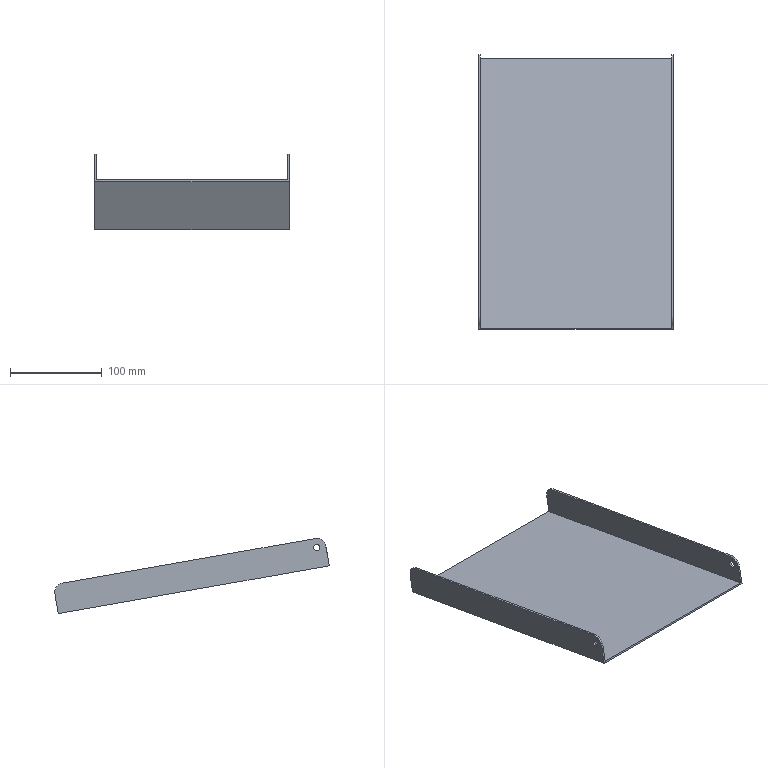Part | NX | features HB 2 | 1 solid | 16 faces | box 213 x 300.028 x 82.132 mm | volume 163815 mm3 | plane 10 | cylinder 6 | commonest cylinder face diameters 20 x4 7 x2
STEP:
#1=CARTESIAN_POINT('',(3721.,686.06,-368.904));
#2=VERTEX_POINT('',#1);
#3=CARTESIAN_POINT('',(3721.,686.966,-372.285));
#4=DIRECTION('',(1.,0.,0.));
#5=DIRECTION('',(0.,-0.2588,0.9659));
#6=AXIS2_PLACEMENT_3D('',#3,#4,#5);
#7=CIRCLE('',#6,3.5);
#8=EDGE_CURVE('',#2,#2,#7,.T.);
#9=ORIENTED_EDGE('',*,*,#8,.T.);
#10=EDGE_LOOP('',(#9));
#11=FACE_BOUND('',#10,.T.);
#12=CARTESIAN_POINT('',(3719.,686.06,-368.904));
#13=VERTEX_POINT('',#12);
#14=CARTESIAN_POINT('',(3719.,686.966,-372.285));
#15=DIRECTION('',(-1.,0.,0.));
#16=DIRECTION('',(0.,-0.2588,0.9659));
#17=AXIS2_PLACEMENT_3D('',#14,#15,#16);
#18=CIRCLE('',#17,3.5);
#19=EDGE_CURVE('',#13,#13,#18,.T.);
#20=ORIENTED_EDGE('',*,*,#19,.T.);
#21=EDGE_LOOP('',(#20));
#22=FACE_BOUND('',#21,.T.);
#23=CARTESIAN_POINT('',(2999.,686.966,-372.285));
#24=DIRECTION('',(1.,0.,0.));
#25=DIRECTION('',(0.,0.2588,-0.9659));
#26=AXIS2_PLACEMENT_3D('',#23,#24,#25);
#27=CYLINDRICAL_SURFACE('',#26,3.5);
#28=ADVANCED_FACE('',(#11,#22),#27,.F.);
#29=CARTESIAN_POINT('',(3721.,965.062,-411.167));
#30=VERTEX_POINT('',#29);
#31=CARTESIAN_POINT('',(3721.,688.702,-362.437));
#32=VERTEX_POINT('',#31);
#33=CARTESIAN_POINT('',(3721.,564.245,-340.492));
#34=DIRECTION('',(0.,-0.9848,0.1736));
#35=VECTOR('',#34,1000.);
#36=LINE('',#33,#35);
#37=EDGE_CURVE('',#30,#32,#36,.T.);
#38=ORIENTED_EDGE('',*,*,#37,.F.);
#39=CARTESIAN_POINT('',(3719.,965.062,-411.167));
#40=VERTEX_POINT('',#39);
#41=CARTESIAN_POINT('',(3605.,965.062,-411.167));
#42=DIRECTION('',(1.,0.,0.));
#43=VECTOR('',#42,1000.);
#44=LINE('',#41,#43);
#45=EDGE_CURVE('',#40,#30,#44,.T.);
#46=ORIENTED_EDGE('',*,*,#45,.F.);
#47=CARTESIAN_POINT('',(3719.,688.702,-362.437));
#48=VERTEX_POINT('',#47);
#49=CARTESIAN_POINT('',(3719.,564.245,-340.492));
#50=DIRECTION('',(0.,-0.9848,0.1736));
#51=VECTOR('',#50,1000.);
#52=LINE('',#49,#51);
#53=EDGE_CURVE('',#40,#48,#52,.T.);
#54=ORIENTED_EDGE('',*,*,#53,.T.);
#55=CARTESIAN_POINT('',(3605.,688.702,-362.437));
#56=DIRECTION('',(1.,0.,0.));
#57=VECTOR('',#56,1000.);
#58=LINE('',#55,#57);
#59=EDGE_CURVE('',#48,#32,#58,.T.);
#60=ORIENTED_EDGE('',*,*,#59,.T.);
#61=EDGE_LOOP('',(#38,#46,#54,#60));
#62=FACE_BOUND('',#61,.T.);
#63=CARTESIAN_POINT('',(3605.,564.245,-340.492));
#64=DIRECTION('',(0.,-0.1736,-0.9848));
#65=DIRECTION('',(0.,0.9848,-0.1736));
#66=AXIS2_PLACEMENT_3D('',#63,#64,#65);
#67=PLANE('',#66);
#68=ADVANCED_FACE('',(#62),#67,.F.);
#69=CARTESIAN_POINT('',(3721.,973.174,-422.751));
#70=VERTEX_POINT('',#69);
#71=CARTESIAN_POINT('',(3721.,963.326,-421.015));
#72=DIRECTION('',(-1.,0.,0.));
#73=DIRECTION('',(0.,-0.2588,0.9659));
#74=AXIS2_PLACEMENT_3D('',#71,#72,#73);
#75=CIRCLE('',#74,10.);
#76=EDGE_CURVE('',#30,#70,#75,.T.);
#77=ORIENTED_EDGE('',*,*,#76,.T.);
#78=CARTESIAN_POINT('',(3719.,973.174,-422.751));
#79=VERTEX_POINT('',#78);
#80=CARTESIAN_POINT('',(3605.,973.174,-422.751));
#81=DIRECTION('',(-1.,0.,0.));
#82=VECTOR('',#81,1000.);
#83=LINE('',#80,#82);
#84=EDGE_CURVE('',#70,#79,#83,.T.);
#85=ORIENTED_EDGE('',*,*,#84,.T.);
#86=CARTESIAN_POINT('',(3719.,963.326,-421.015));
#87=DIRECTION('',(1.,0.,0.));
#88=DIRECTION('',(0.,-0.2588,0.9659));
#89=AXIS2_PLACEMENT_3D('',#86,#87,#88);
#90=CIRCLE('',#89,10.);
#91=EDGE_CURVE('',#79,#40,#90,.T.);
#92=ORIENTED_EDGE('',*,*,#91,.T.);
#93=ORIENTED_EDGE('',*,*,#45,.T.);
#94=EDGE_LOOP('',(#77,#85,#92,#93));
#95=FACE_BOUND('',#94,.T.);
#96=CARTESIAN_POINT('',(3605.,963.326,-421.015));
#97=DIRECTION('',(-1.,0.,0.));
#98=DIRECTION('',(0.,-0.2588,0.9659));
#99=AXIS2_PLACEMENT_3D('',#96,#97,#98);
#100=CYLINDRICAL_SURFACE('',#99,10.);
#101=ADVANCED_FACE('',(#95),#100,.T.);
#102=ORIENTED_EDGE('',*,*,#53,.F.);
#103=ORIENTED_EDGE('',*,*,#91,.F.);
#104=CARTESIAN_POINT('',(3719.,969.354,-444.417));
#105=VERTEX_POINT('',#104);
#106=CARTESIAN_POINT('',(3719.,969.701,-442.448));
#107=DIRECTION('',(0.,0.1736,0.9848));
#108=VECTOR('',#107,1000.);
#109=LINE('',#106,#108);
#110=EDGE_CURVE('',#105,#79,#109,.T.);
#111=ORIENTED_EDGE('',*,*,#110,.F.);
#112=CARTESIAN_POINT('',(3719.,673.298,-392.215));
#113=VERTEX_POINT('',#112);
#114=CARTESIAN_POINT('',(3719.,558.689,-372.006));
#115=DIRECTION('',(0.,0.9848,-0.1736));
#116=VECTOR('',#115,1000.);
#117=LINE('',#114,#116);
#118=EDGE_CURVE('',#113,#105,#117,.T.);
#119=ORIENTED_EDGE('',*,*,#118,.F.);
#120=CARTESIAN_POINT('',(3719.,677.118,-370.549));
#121=VERTEX_POINT('',#120);
#122=CARTESIAN_POINT('',(3719.,673.645,-390.245));
#123=DIRECTION('',(0.,0.1736,0.9848));
#124=VECTOR('',#123,1000.);
#125=LINE('',#122,#124);
#126=EDGE_CURVE('',#113,#121,#125,.T.);
#127=ORIENTED_EDGE('',*,*,#126,.T.);
#128=CARTESIAN_POINT('',(3719.,686.966,-372.285));
#129=DIRECTION('',(-1.,0.,0.));
#130=DIRECTION('',(0.,0.5736,0.8192));
#131=AXIS2_PLACEMENT_3D('',#128,#129,#130);
#132=CIRCLE('',#131,10.);
#133=EDGE_CURVE('',#121,#48,#132,.T.);
#134=ORIENTED_EDGE('',*,*,#133,.T.);
#135=EDGE_LOOP('',(#102,#103,#111,#119,#127,#134));
#136=FACE_BOUND('',#135,.T.);
#137=ORIENTED_EDGE('',*,*,#19,.F.);
#138=EDGE_LOOP('',(#137));
#139=FACE_BOUND('',#138,.T.);
#140=CARTESIAN_POINT('',(3719.,559.036,-370.036));
#141=DIRECTION('',(1.,0.,0.));
#142=DIRECTION('',(0.,0.2588,-0.9659));
#143=AXIS2_PLACEMENT_3D('',#140,#141,#142);
#144=PLANE('',#143);
#145=ADVANCED_FACE('',(#136,#139),#144,.F.);
#146=CARTESIAN_POINT('',(3721.,677.118,-370.549));
#147=VERTEX_POINT('',#146);
#148=CARTESIAN_POINT('',(3721.,686.966,-372.285));
#149=DIRECTION('',(1.,0.,0.));
#150=DIRECTION('',(0.,0.5736,0.8192));
#151=AXIS2_PLACEMENT_3D('',#148,#149,#150);
#152=CIRCLE('',#151,10.);
#153=EDGE_CURVE('',#32,#147,#152,.T.);
#154=ORIENTED_EDGE('',*,*,#153,.F.);
#155=ORIENTED_EDGE('',*,*,#59,.F.);
#156=ORIENTED_EDGE('',*,*,#133,.F.);
#157=CARTESIAN_POINT('',(3700.,677.118,-370.549));
#158=DIRECTION('',(-1.,0.,0.));
#159=VECTOR('',#158,1000.);
#160=LINE('',#157,#159);
#161=EDGE_CURVE('',#147,#121,#160,.T.);
#162=ORIENTED_EDGE('',*,*,#161,.F.);
#163=EDGE_LOOP('',(#154,#155,#156,#162));
#164=FACE_BOUND('',#163,.T.);
#165=CARTESIAN_POINT('',(3605.,686.966,-372.285));
#166=DIRECTION('',(-1.,0.,0.));
#167=DIRECTION('',(0.,0.5736,0.8192));
#168=AXIS2_PLACEMENT_3D('',#165,#166,#167);
#169=CYLINDRICAL_SURFACE('',#168,10.);
#170=ADVANCED_FACE('',(#164),#169,.T.);
#171=ORIENTED_EDGE('',*,*,#76,.F.);
#172=ORIENTED_EDGE('',*,*,#37,.T.);
#173=ORIENTED_EDGE('',*,*,#153,.T.);
#174=CARTESIAN_POINT('',(3721.,673.645,-390.245));
#175=VERTEX_POINT('',#174);
#176=CARTESIAN_POINT('',(3721.,673.645,-390.245));
#177=DIRECTION('',(0.,0.1736,0.9848));
#178=VECTOR('',#177,1000.);
#179=LINE('',#176,#178);
#180=EDGE_CURVE('',#175,#147,#179,.T.);
#181=ORIENTED_EDGE('',*,*,#180,.F.);
#182=CARTESIAN_POINT('',(3721.,969.701,-442.448));
#183=VERTEX_POINT('',#182);
#184=CARTESIAN_POINT('',(3721.,559.036,-370.036));
#185=DIRECTION('',(0.,-0.9848,0.1736));
#186=VECTOR('',#185,1000.);
#187=LINE('',#184,#186);
#188=EDGE_CURVE('',#183,#175,#187,.T.);
#189=ORIENTED_EDGE('',*,*,#188,.F.);
#190=CARTESIAN_POINT('',(3721.,969.701,-442.448));
#191=DIRECTION('',(0.,0.1736,0.9848));
#192=VECTOR('',#191,1000.);
#193=LINE('',#190,#192);
#194=EDGE_CURVE('',#183,#70,#193,.T.);
#195=ORIENTED_EDGE('',*,*,#194,.T.);
#196=EDGE_LOOP('',(#171,#172,#173,#181,#189,#195));
#197=FACE_BOUND('',#196,.T.);
#198=ORIENTED_EDGE('',*,*,#8,.F.);
#199=EDGE_LOOP('',(#198));
#200=FACE_BOUND('',#199,.T.);
#201=CARTESIAN_POINT('',(3721.,559.036,-370.036));
#202=DIRECTION('',(1.,0.,0.));
#203=DIRECTION('',(0.,-0.2588,0.9659));
#204=AXIS2_PLACEMENT_3D('',#201,#202,#203);
#205=PLANE('',#204);
#206=ADVANCED_FACE('',(#197,#200),#205,.T.);
#207=CARTESIAN_POINT('',(3930.,673.645,-390.245));
#208=VERTEX_POINT('',#207);
#209=CARTESIAN_POINT('',(3700.,673.645,-390.245));
#210=DIRECTION('',(1.,0.,0.));
#211=VECTOR('',#210,1000.);
#212=LINE('',#209,#211);
#213=EDGE_CURVE('',#175,#208,#212,.T.);
#214=ORIENTED_EDGE('',*,*,#213,.F.);
#215=ORIENTED_EDGE('',*,*,#180,.T.);
#216=ORIENTED_EDGE('',*,*,#161,.T.);
#217=ORIENTED_EDGE('',*,*,#126,.F.);
#218=CARTESIAN_POINT('',(3932.,673.298,-392.215));
#219=VERTEX_POINT('',#218);
#220=CARTESIAN_POINT('',(3700.,673.298,-392.215));
#221=DIRECTION('',(1.,0.,0.));
#222=VECTOR('',#221,1000.);
#223=LINE('',#220,#222);
#224=EDGE_CURVE('',#113,#219,#223,.T.);
#225=ORIENTED_EDGE('',*,*,#224,.T.);
#226=CARTESIAN_POINT('',(3932.,677.118,-370.549));
#227=VERTEX_POINT('',#226);
#228=CARTESIAN_POINT('',(3932.,673.645,-390.245));
#229=DIRECTION('',(0.,0.1736,0.9848));
#230=VECTOR('',#229,1000.);
#231=LINE('',#228,#230);
#232=EDGE_CURVE('',#219,#227,#231,.T.);
#233=ORIENTED_EDGE('',*,*,#232,.T.);
#234=CARTESIAN_POINT('',(3930.,677.118,-370.549));
#235=VERTEX_POINT('',#234);
#236=CARTESIAN_POINT('',(3619.,677.118,-370.549));
#237=DIRECTION('',(-1.,0.,0.));
#238=VECTOR('',#237,1000.);
#239=LINE('',#236,#238);
#240=EDGE_CURVE('',#227,#235,#239,.T.);
#241=ORIENTED_EDGE('',*,*,#240,.T.);
#242=CARTESIAN_POINT('',(3930.,673.645,-390.245));
#243=DIRECTION('',(0.,0.1736,0.9848));
#244=VECTOR('',#243,1000.);
#245=LINE('',#242,#244);
#246=EDGE_CURVE('',#208,#235,#245,.T.);
#247=ORIENTED_EDGE('',*,*,#246,.F.);
#248=EDGE_LOOP('',(#214,#215,#216,#217,#225,#233,#241,#247));
#249=FACE_BOUND('',#248,.T.);
#250=CARTESIAN_POINT('',(3700.,673.645,-390.245));
#251=DIRECTION('',(0.,0.9848,-0.1736));
#252=DIRECTION('',(0.,-0.1736,-0.9848));
#253=AXIS2_PLACEMENT_3D('',#250,#251,#252);
#254=PLANE('',#253);
#255=ADVANCED_FACE('',(#249),#254,.F.);
#256=ORIENTED_EDGE('',*,*,#194,.F.);
#257=CARTESIAN_POINT('',(3930.,969.701,-442.448));
#258=VERTEX_POINT('',#257);
#259=CARTESIAN_POINT('',(3700.,969.701,-442.448));
#260=DIRECTION('',(1.,0.,0.));
#261=VECTOR('',#260,1000.);
#262=LINE('',#259,#261);
#263=EDGE_CURVE('',#183,#258,#262,.T.);
#264=ORIENTED_EDGE('',*,*,#263,.T.);
#265=CARTESIAN_POINT('',(3930.,973.174,-422.751));
#266=VERTEX_POINT('',#265);
#267=CARTESIAN_POINT('',(3930.,969.701,-442.448));
#268=DIRECTION('',(0.,0.1736,0.9848));
#269=VECTOR('',#268,1000.);
#270=LINE('',#267,#269);
#271=EDGE_CURVE('',#258,#266,#270,.T.);
#272=ORIENTED_EDGE('',*,*,#271,.T.);
#273=CARTESIAN_POINT('',(3932.,973.174,-422.751));
#274=VERTEX_POINT('',#273);
#275=CARTESIAN_POINT('',(3645.,973.174,-422.751));
#276=DIRECTION('',(-1.,0.,0.));
#277=VECTOR('',#276,1000.);
#278=LINE('',#275,#277);
#279=EDGE_CURVE('',#274,#266,#278,.T.);
#280=ORIENTED_EDGE('',*,*,#279,.F.);
#281=CARTESIAN_POINT('',(3932.,969.354,-444.417));
#282=VERTEX_POINT('',#281);
#283=CARTESIAN_POINT('',(3932.,969.701,-442.448));
#284=DIRECTION('',(0.,0.1736,0.9848));
#285=VECTOR('',#284,1000.);
#286=LINE('',#283,#285);
#287=EDGE_CURVE('',#282,#274,#286,.T.);
#288=ORIENTED_EDGE('',*,*,#287,.F.);
#289=CARTESIAN_POINT('',(3700.,969.354,-444.417));
#290=DIRECTION('',(1.,0.,0.));
#291=VECTOR('',#290,1000.);
#292=LINE('',#289,#291);
#293=EDGE_CURVE('',#105,#282,#292,.T.);
#294=ORIENTED_EDGE('',*,*,#293,.F.);
#295=ORIENTED_EDGE('',*,*,#110,.T.);
#296=ORIENTED_EDGE('',*,*,#84,.F.);
#297=EDGE_LOOP('',(#256,#264,#272,#280,#288,#294,#295,#296));
#298=FACE_BOUND('',#297,.T.);
#299=CARTESIAN_POINT('',(3700.,969.701,-442.448));
#300=DIRECTION('',(0.,-0.9848,0.1736));
#301=DIRECTION('',(0.,-0.1736,-0.9848));
#302=AXIS2_PLACEMENT_3D('',#299,#300,#301);
#303=PLANE('',#302);
#304=ADVANCED_FACE('',(#298),#303,.F.);
#305=ORIENTED_EDGE('',*,*,#118,.T.);
#306=ORIENTED_EDGE('',*,*,#293,.T.);
#307=CARTESIAN_POINT('',(3932.,558.689,-372.006));
#308=DIRECTION('',(0.,-0.9848,0.1736));
#309=VECTOR('',#308,1000.);
#310=LINE('',#307,#309);
#311=EDGE_CURVE('',#282,#219,#310,.T.);
#312=ORIENTED_EDGE('',*,*,#311,.T.);
#313=ORIENTED_EDGE('',*,*,#224,.F.);
#314=EDGE_LOOP('',(#305,#306,#312,#313));
#315=FACE_BOUND('',#314,.T.);
#316=CARTESIAN_POINT('',(3700.,558.689,-372.006));
#317=DIRECTION('',(0.,0.1736,0.9848));
#318=DIRECTION('',(1.,0.,0.));
#319=AXIS2_PLACEMENT_3D('',#316,#317,#318);
#320=PLANE('',#319);
#321=ADVANCED_FACE('',(#315),#320,.F.);
#322=ORIENTED_EDGE('',*,*,#263,.F.);
#323=ORIENTED_EDGE('',*,*,#188,.T.);
#324=ORIENTED_EDGE('',*,*,#213,.T.);
#325=CARTESIAN_POINT('',(3930.,559.036,-370.036));
#326=DIRECTION('',(0.,0.9848,-0.1736));
#327=VECTOR('',#326,1000.);
#328=LINE('',#325,#327);
#329=EDGE_CURVE('',#208,#258,#328,.T.);
#330=ORIENTED_EDGE('',*,*,#329,.T.);
#331=EDGE_LOOP('',(#322,#323,#324,#330));
#332=FACE_BOUND('',#331,.T.);
#333=CARTESIAN_POINT('',(3700.,559.036,-370.036));
#334=DIRECTION('',(0.,0.1736,0.9848));
#335=DIRECTION('',(1.,0.,0.));
#336=AXIS2_PLACEMENT_3D('',#333,#334,#335);
#337=PLANE('',#336);
#338=ADVANCED_FACE('',(#332),#337,.T.);
#339=CARTESIAN_POINT('',(3932.,687.872,-375.666));
#340=VERTEX_POINT('',#339);
#341=CARTESIAN_POINT('',(3932.,686.966,-372.285));
#342=DIRECTION('',(1.,0.,0.));
#343=DIRECTION('',(0.,0.2588,-0.9659));
#344=AXIS2_PLACEMENT_3D('',#341,#342,#343);
#345=CIRCLE('',#344,3.5);
#346=EDGE_CURVE('',#340,#340,#345,.T.);
#347=ORIENTED_EDGE('',*,*,#346,.F.);
#348=EDGE_LOOP('',(#347));
#349=FACE_BOUND('',#348,.T.);
#350=ORIENTED_EDGE('',*,*,#311,.F.);
#351=ORIENTED_EDGE('',*,*,#287,.T.);
#352=CARTESIAN_POINT('',(3932.,965.062,-411.167));
#353=VERTEX_POINT('',#352);
#354=CARTESIAN_POINT('',(3932.,963.326,-421.015));
#355=DIRECTION('',(-1.,0.,0.));
#356=DIRECTION('',(0.,0.2588,-0.9659));
#357=AXIS2_PLACEMENT_3D('',#354,#355,#356);
#358=CIRCLE('',#357,10.);
#359=EDGE_CURVE('',#353,#274,#358,.T.);
#360=ORIENTED_EDGE('',*,*,#359,.F.);
#361=CARTESIAN_POINT('',(3932.,688.702,-362.437));
#362=VERTEX_POINT('',#361);
#363=CARTESIAN_POINT('',(3932.,564.245,-340.492));
#364=DIRECTION('',(0.,-0.9848,0.1736));
#365=VECTOR('',#364,1000.);
#366=LINE('',#363,#365);
#367=EDGE_CURVE('',#353,#362,#366,.T.);
#368=ORIENTED_EDGE('',*,*,#367,.T.);
#369=CARTESIAN_POINT('',(3932.,686.966,-372.285));
#370=DIRECTION('',(1.,0.,0.));
#371=DIRECTION('',(0.,-0.5736,-0.8192));
#372=AXIS2_PLACEMENT_3D('',#369,#370,#371);
#373=CIRCLE('',#372,10.);
#374=EDGE_CURVE('',#362,#227,#373,.T.);
#375=ORIENTED_EDGE('',*,*,#374,.T.);
#376=ORIENTED_EDGE('',*,*,#232,.F.);
#377=EDGE_LOOP('',(#350,#351,#360,#368,#375,#376));
#378=FACE_BOUND('',#377,.T.);
#379=CARTESIAN_POINT('',(3932.,559.036,-370.036));
#380=DIRECTION('',(-1.,0.,0.));
#381=DIRECTION('',(0.,-0.2588,0.9659));
#382=AXIS2_PLACEMENT_3D('',#379,#380,#381);
#383=PLANE('',#382);
#384=ADVANCED_FACE('',(#349,#378),#383,.F.);
#385=ORIENTED_EDGE('',*,*,#367,.F.);
#386=CARTESIAN_POINT('',(3930.,965.062,-411.167));
#387=VERTEX_POINT('',#386);
#388=CARTESIAN_POINT('',(3877.,965.062,-411.167));
#389=DIRECTION('',(1.,0.,0.));
#390=VECTOR('',#389,1000.);
#391=LINE('',#388,#390);
#392=EDGE_CURVE('',#387,#353,#391,.T.);
#393=ORIENTED_EDGE('',*,*,#392,.F.);
#394=CARTESIAN_POINT('',(3930.,688.702,-362.437));
#395=VERTEX_POINT('',#394);
#396=CARTESIAN_POINT('',(3930.,564.245,-340.492));
#397=DIRECTION('',(0.,-0.9848,0.1736));
#398=VECTOR('',#397,1000.);
#399=LINE('',#396,#398);
#400=EDGE_CURVE('',#387,#395,#399,.T.);
#401=ORIENTED_EDGE('',*,*,#400,.T.);
#402=CARTESIAN_POINT('',(3877.,688.702,-362.437));
#403=DIRECTION('',(1.,0.,0.));
#404=VECTOR('',#403,1000.);
#405=LINE('',#402,#404);
#406=EDGE_CURVE('',#395,#362,#405,.T.);
#407=ORIENTED_EDGE('',*,*,#406,.T.);
#408=EDGE_LOOP('',(#385,#393,#401,#407));
#409=FACE_BOUND('',#408,.T.);
#410=CARTESIAN_POINT('',(3877.,564.245,-340.492));
#411=DIRECTION('',(0.,-0.1736,-0.9848));
#412=DIRECTION('',(0.,0.9848,-0.1736));
#413=AXIS2_PLACEMENT_3D('',#410,#411,#412);
#414=PLANE('',#413);
#415=ADVANCED_FACE('',(#409),#414,.F.);
#416=CARTESIAN_POINT('',(3930.,687.872,-375.666));
#417=VERTEX_POINT('',#416);
#418=CARTESIAN_POINT('',(3930.,686.966,-372.285));
#419=DIRECTION('',(1.,0.,0.));
#420=DIRECTION('',(0.,0.2588,-0.9659));
#421=AXIS2_PLACEMENT_3D('',#418,#419,#420);
#422=CIRCLE('',#421,3.5);
#423=EDGE_CURVE('',#417,#417,#422,.T.);
#424=ORIENTED_EDGE('',*,*,#423,.T.);
#425=EDGE_LOOP('',(#424));
#426=FACE_BOUND('',#425,.T.);
#427=ORIENTED_EDGE('',*,*,#329,.F.);
#428=ORIENTED_EDGE('',*,*,#246,.T.);
#429=CARTESIAN_POINT('',(3930.,686.966,-372.285));
#430=DIRECTION('',(-1.,0.,0.));
#431=DIRECTION('',(0.,-0.5736,-0.8192));
#432=AXIS2_PLACEMENT_3D('',#429,#430,#431);
#433=CIRCLE('',#432,10.);
#434=EDGE_CURVE('',#235,#395,#433,.T.);
#435=ORIENTED_EDGE('',*,*,#434,.T.);
#436=ORIENTED_EDGE('',*,*,#400,.F.);
#437=CARTESIAN_POINT('',(3930.,963.326,-421.015));
#438=DIRECTION('',(1.,0.,0.));
#439=DIRECTION('',(0.,0.2588,-0.9659));
#440=AXIS2_PLACEMENT_3D('',#437,#438,#439);
#441=CIRCLE('',#440,10.);
#442=EDGE_CURVE('',#266,#387,#441,.T.);
#443=ORIENTED_EDGE('',*,*,#442,.F.);
#444=ORIENTED_EDGE('',*,*,#271,.F.);
#445=EDGE_LOOP('',(#427,#428,#435,#436,#443,#444));
#446=FACE_BOUND('',#445,.T.);
#447=CARTESIAN_POINT('',(3930.,559.036,-370.036));
#448=DIRECTION('',(-1.,0.,0.));
#449=DIRECTION('',(0.,-0.2588,0.9659));
#450=AXIS2_PLACEMENT_3D('',#447,#448,#449);
#451=PLANE('',#450);
#452=ADVANCED_FACE('',(#426,#446),#451,.T.);
#453=ORIENTED_EDGE('',*,*,#442,.T.);
#454=ORIENTED_EDGE('',*,*,#392,.T.);
#455=ORIENTED_EDGE('',*,*,#359,.T.);
#456=ORIENTED_EDGE('',*,*,#279,.T.);
#457=EDGE_LOOP('',(#453,#454,#455,#456));
#458=FACE_BOUND('',#457,.T.);
#459=CARTESIAN_POINT('',(3619.,963.326,-421.015));
#460=DIRECTION('',(1.,0.,0.));
#461=DIRECTION('',(0.,0.2588,-0.9659));
#462=AXIS2_PLACEMENT_3D('',#459,#460,#461);
#463=CYLINDRICAL_SURFACE('',#462,10.);
#464=ADVANCED_FACE('',(#458),#463,.T.);
#465=ORIENTED_EDGE('',*,*,#434,.F.);
#466=ORIENTED_EDGE('',*,*,#240,.F.);
#467=ORIENTED_EDGE('',*,*,#374,.F.);
#468=ORIENTED_EDGE('',*,*,#406,.F.);
#469=EDGE_LOOP('',(#465,#466,#467,#468));
#470=FACE_BOUND('',#469,.T.);
#471=CARTESIAN_POINT('',(3619.,686.966,-372.285));
#472=DIRECTION('',(1.,0.,0.));
#473=DIRECTION('',(0.,-0.5736,-0.8192));
#474=AXIS2_PLACEMENT_3D('',#471,#472,#473);
#475=CYLINDRICAL_SURFACE('',#474,10.);
#476=ADVANCED_FACE('',(#470),#475,.T.);
#477=ORIENTED_EDGE('',*,*,#423,.F.);
#478=EDGE_LOOP('',(#477));
#479=FACE_BOUND('',#478,.T.);
#480=ORIENTED_EDGE('',*,*,#346,.T.);
#481=EDGE_LOOP('',(#480));
#482=FACE_BOUND('',#481,.T.);
#483=CARTESIAN_POINT('',(3879.,686.966,-372.285));
#484=DIRECTION('',(-1.,0.,0.));
#485=DIRECTION('',(0.,-0.2588,0.9659));
#486=AXIS2_PLACEMENT_3D('',#483,#484,#485);
#487=CYLINDRICAL_SURFACE('',#486,3.5);
#488=ADVANCED_FACE('',(#479,#482),#487,.F.);
#489=CLOSED_SHELL('',(#28,#68,#101,#145,#170,#206,#255,#304,#321,#338,#384,#415,#452,#464,#476,#488));
#490=MANIFOLD_SOLID_BREP('',#489);
#491=(LENGTH_UNIT()NAMED_UNIT(*)SI_UNIT(.MILLI.,.METRE.));
#492=UNCERTAINTY_MEASURE_WITH_UNIT(LENGTH_MEASURE(0.00001),#491,'','');
#493=(NAMED_UNIT(*)PLANE_ANGLE_UNIT()SI_UNIT($,.RADIAN.));
#494=(NAMED_UNIT(*)SI_UNIT($,.STERADIAN.)SOLID_ANGLE_UNIT());
#495=(GEOMETRIC_REPRESENTATION_CONTEXT(3)GLOBAL_UNCERTAINTY_ASSIGNED_CONTEXT((#492))GLOBAL_UNIT_ASSIGNED_CONTEXT((#491,#493,#494))REPRESENTATION_CONTEXT('',''));
#496=ADVANCED_BREP_SHAPE_REPRESENTATION('',(#490),#495);